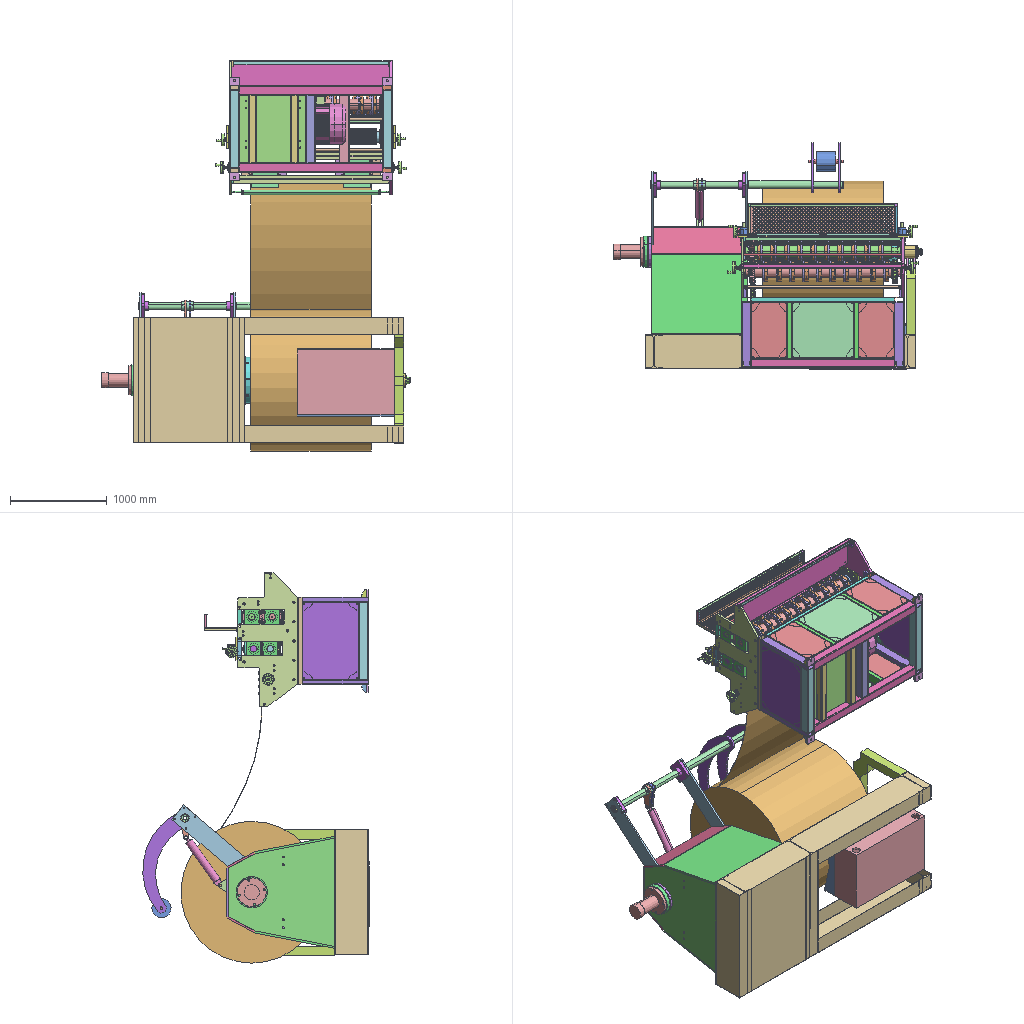Assembly | SolidWorks | 136 different items | 508 placed | box 3192 x 2340 x 4038 mm
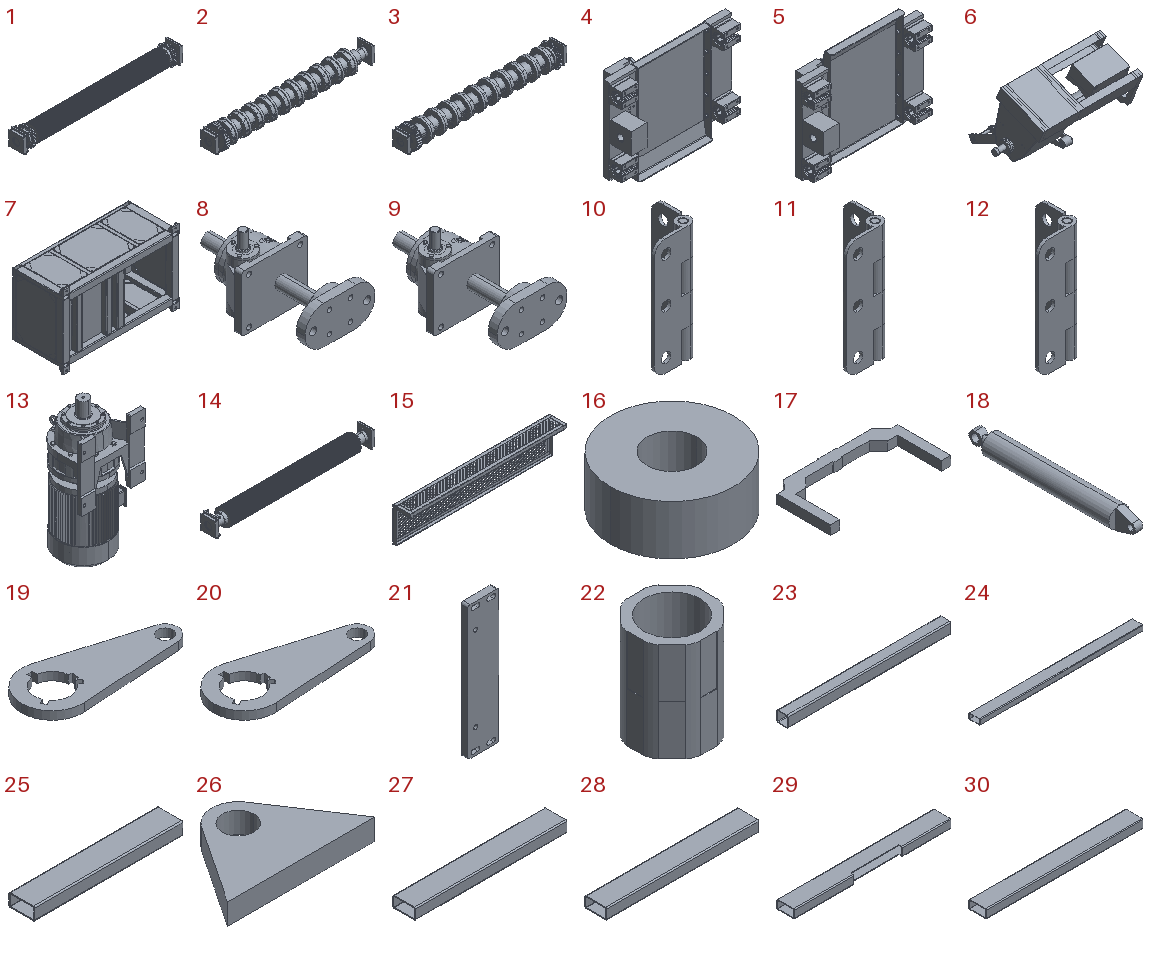Parts list (item | name | quantity | parent item | size | volume | features):
1 | (subassembly) | x1 | - | 1672 x 198.631 x 197.926 mm | 35053418 mm3 | -
2 | (subassembly) | x1 | - | 1672 x 223.661 x 223.999 mm | 30966531 mm3 | -
3 | (subassembly) | x1 | - | 1672 x 235.877 x 235.04 mm | 32005063 mm3 | -
4 | (subassembly) | x1 | - | - | 3227627 mm3 | -
5 | (subassembly) | x1 | - | - | 3227627 mm3 | -
6 | (subassembly) | x1 | - | - | 464591008 mm3 | -
7 | (subassembly) | x1 | - | 1682 x 730 x 1060 mm | 39110385 mm3 | -
8 | (subassembly) | x1 | - | 138.5 x 246 x 160 mm | 888855 mm3 | -
9 | (subassembly) | x1 | - | 138.5 x 246 x 160 mm | 888855 mm3 | -
10 | (subassembly) | x1 | - | 28.6 x 28.6 x 78 mm | 10885 mm3 | -
11 | (subassembly) | x1 | - | 28.6 x 28.6 x 78 mm | 10885 mm3 | -
12 | (subassembly) | x1 | - | 28.6 x 28.6 x 78 mm | 10885 mm3 | -
13 | (subassembly) | x1 | - | 570 x 540.12 x 1100 mm | 120754101 mm3 | -
14 | (subassembly) | x1 | - | 1672 x 169.976 x 180 mm | 33756798 mm3 | -
15 | - | x1 | - | - | 1424009 mm3 | features BaseBody 11
16 | - | x4 | in 6 | 49.497 x 49.497 x 20 mm | 32201 mm3 | features BaseBody 1
17 | - | x1 | in 6 | 1310 x 690 x 100 mm | 25394673 mm3 | features BaseBody 1
18 | - | x1 | in 6 | 80 x 654.288 x 80 mm | 2684074 mm3 | features BaseBody 1
19 | - | x1 | in 6 | 283.692 x 120 x 16 mm | 303267 mm3 | features BaseBody 1
20 | - | x1 | in 6 | 283.692 x 120 x 16 mm | 303267 mm3 | features BaseBody 1
21 | - | x2 | - | 140 x 30 x 600 mm | 2424100 mm3 | features BaseBody 1
22 | - | x1 | in 6 | 224.499 x 224.499 x 300 mm | 5216561 mm3 | features BaseBody 1
23 | - | x2 | in 7 | 1480 x 100 x 100 mm | 2716717 mm3 | features BaseBody 1
24 | - | x2 | in 7 | 1480 x 100 x 50 mm | 1650789 mm3 | features BaseBody 1
25 | - | x4 | in 7 | 580 x 100 x 50 mm | 646931 mm3 | features BaseBody 1
26 | - | x2 | in 6 | 140 x 85 x 20 mm | 126524 mm3 | features BaseBody 1
27 | - | x4 | in 7 | 680 x 100 x 50 mm | 758471 mm3 | features BaseBody 1
28 | - | x2 | in 7 | 700 x 100 x 50 mm | 780779 mm3 | features BaseBody 1
29 | - | x1 | in 7 | 900 x 100 x 50 mm | 914903 mm3 | features BaseBody 1
30 | - | x1 | in 7 | 900 x 100 x 50 mm | 1003858 mm3 | features BaseBody 1
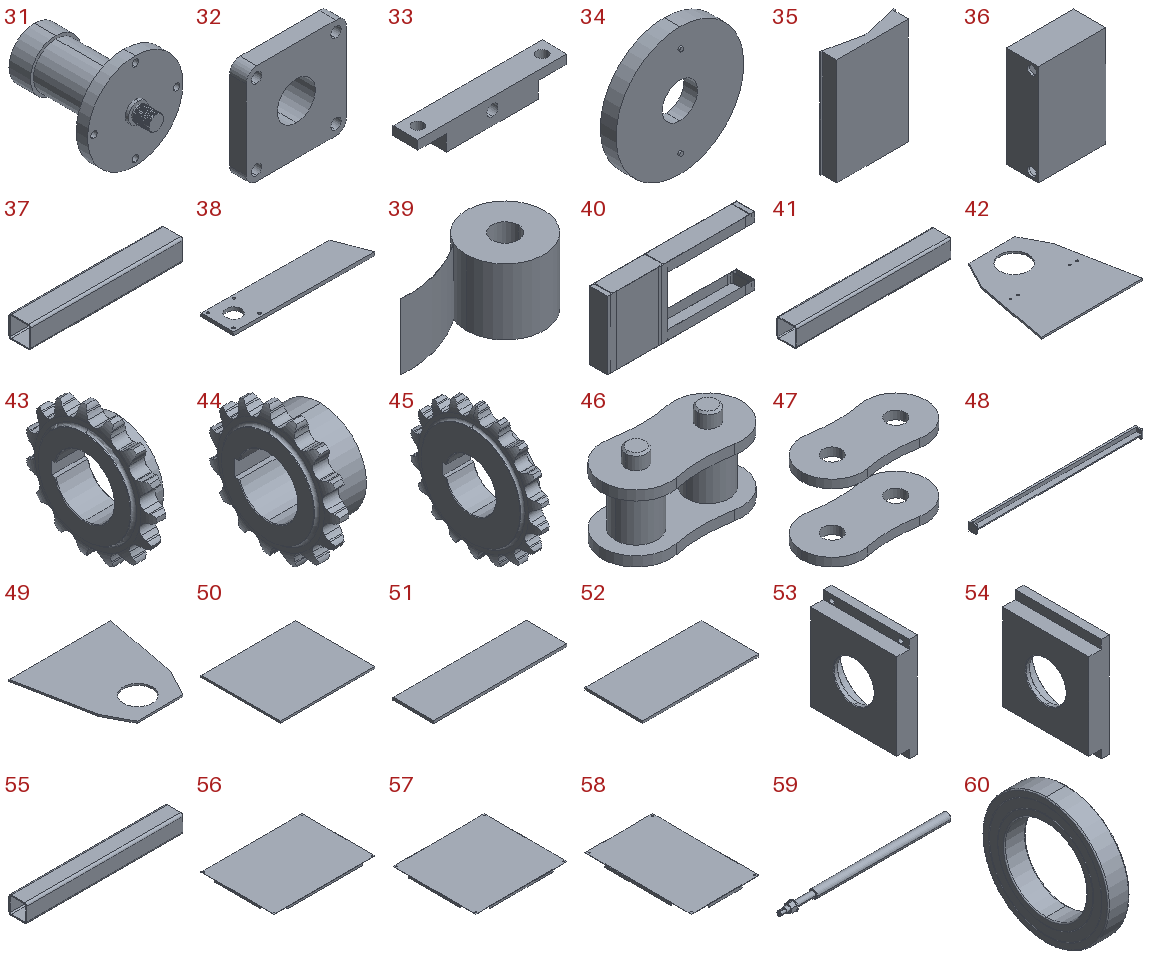31 | - | x1 | in 6 | 300 x 382.79 x 300 mm | 7334262 mm3 | features BaseBody 1
32 | - | x2 | in 6 | 193 x 74.6 x 193 mm | 1117041 mm3 | features BaseBody 1
33 | - | x2 | - | 240 x 40 x 40 mm | 271016 mm3 | features BaseBody 1
34 | - | x1 | in 6 | 325 x 45 x 325 mm | 2743003 mm3 | features BaseBody 1
35 | - | x1 | in 6 | 698.157 x 148.827 x 1000 mm | 73538698 mm3 | features BaseBody 1
36 | - | x1 | in 6 | 670 x 320 x 1000 mm | 50005072 mm3 | features BaseBody 1
37 | - | x1 | in 7 | 700 x 100 x 100 mm | 1284934 mm3 | features BaseBody 1
38 | - | x2 | in 6 | 828.827 x 200.894 x 20 mm | 2911165 mm3 | features BaseBody 1
39 | - | x1 | - | 2820 x 1466 x 1250 mm | 1870768700 mm3 | features ExtruThin 1, ICE 1
40 | - | x1 | in 6 | 2800 x 350 x 1296 mm | 23944279 mm3 | features BaseBody 1
41 | - | x2 | in 7 | 800 x 100 x 100 mm | 1468496 mm3 | features BaseBody 1
42 | - | x1 | in 6 | 1120 x 1100 x 20 mm | 17817233 mm3 | features BaseBody 1
43 | - | x2 | in 1 | 50 x 197.46 x 198.492 mm | 656500 mm3 | features BaseBody 1
44 | - | x1 | - | 80 x 197.46 x 198.492 mm | 920770 mm3 | features BaseBody 1
45 | - | x1 | in 3 | 50 x 233.402 x 236 mm | 1046718 mm3 | features BaseBody 1
46 | - | x41 | - | 74.3 x 36.2 x 50.8 mm | 46286 mm3 | features BaseBody 1
47 | - | x41 | - | 74.3 x 36.2 x 45.44 mm | 21265 mm3 | features BaseBody 2
48 | - | x2 | - | 1632 x 70 x 80 mm | 3525010 mm3 | features BaseBody 4
49 | - | x1 | in 6 | 1120 x 1100 x 20 mm | 17842366 mm3 | features BaseBody 1
50 | - | x2 | in 6 | 1000 x 836 x 20 mm | 16720000 mm3 | features BaseBody 1
51 | - | x2 | in 6 | 1000 x 305 x 20 mm | 6100000 mm3 | features BaseBody 1
52 | - | x1 | in 6 | 1000 x 500 x 20 mm | 10000000 mm3 | features BaseBody 1
53 | - | x4 | in 1, 2, 3, 14 | 36 x 150 x 180 mm | 519040 mm3 | features BaseBody 1
54 | - | x4 | in 1, 2, 3, 14 | 36 x 150 x 180 mm | 522217 mm3 | features BaseBody 1
55 | - | x2 | in 7 | 700 x 80 x 80 mm | 1004934 mm3 | features BaseBody 1
56 | - | x2 | in 7 | 795 x 575 x 15 mm | 579015 mm3 | features BaseBody 1
57 | - | x2 | in 7 | 635 x 575 x 15 mm | 463497 mm3 | features BaseBody 1
58 | - | x4 | in 7 | 365 x 575 x 15 mm | 268880 mm3 | features BaseBody 1
59 | - | x2 | - | 527.001 x 30 x 30 mm | 250409 mm3 | features BaseBody 3
60 | - | x2 | in 6 | 22 x 130 x 130 mm | 128128 mm3 | features BaseBody 26
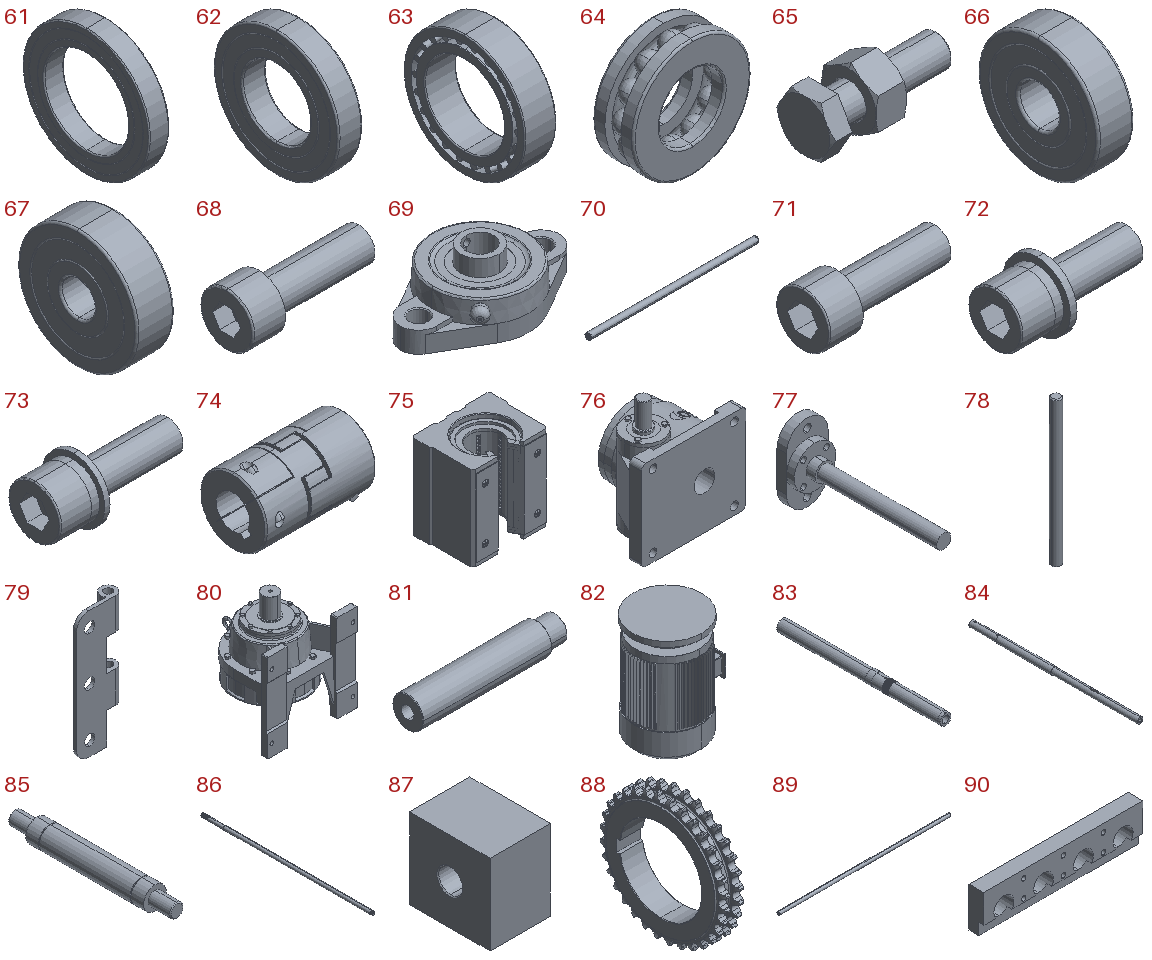61 | - | x1 | in 6 | 38 x 240 x 240 mm | 735391 mm3 | features BaseBody 27
62 | - | x8 | in 1, 2, 3, 14 | 23 x 120 x 120 mm | 144421 mm3 | features BaseBody 19
63 | - | x1 | in 6 | 67 x 260 x 260 mm | 1601339 mm3 | features BaseBody 1
64 | - | x2 | - | 35 x 12 x 35 mm | 6237 mm3 | features BaseBody 1
65 | - | x16 | in 1, 2, 3, 14 | 41.4 x 18.475 x 19.63 mm | 5747 mm3 | features BaseBody 2
66 | - | x20 | in 4, 5 | 9 x 30 x 30 mm | 4389 mm3 | features BaseBody 12
67 | - | x8 | in 4, 5 | 11 x 35 x 35 mm | 7523 mm3 | features BaseBody 11
68 | - | x44 | in 4, 5 | 33 x 13 x 13 mm | 2188 mm3 | features BaseBody 1
69 | - | x2 | - | 99 x 61 x 32.9 mm | 54285 mm3 | features BaseBody 1
70 | - | x1 | - | 1429 x 50 x 50 mm | 1432811 mm3 | features BaseBody 21
71 | - | x8 | in 4, 5 | 40 x 16 x 16 mm | 4026 mm3 | features BaseBody 1
72 | - | x8 | in 4, 5 | 40 x 20 x 20 mm | 4745 mm3 | features BaseBody 3
73 | - | x20 | in 4, 5 | 26 x 12 x 12 mm | 1103 mm3 | features BaseBody 3
74 | - | x2 | - | 66 x 41.729 x 41.508 mm | 63397 mm3 | features BaseBody 3
75 | - | x8 | in 4, 5 | 60 x 47.265 x 65 mm | 129093 mm3 | features BaseBody 5
76 | - | x2 | in 8, 9 | 122 x 84 x 160 mm | 620061 mm3 | features BaseBody 1
77 | - | x2 | in 8, 9 | 70 x 246 x 130 mm | 268794 mm3 | features BaseBody 3
78 | - | x3 | in 10, 11, 12 | 5 x 5 x 78 mm | 1528 mm3 | features BaseBody 1
79 | - | x6 | in 10, 11, 12 | 28.6 x 9.2 x 78 mm | 4679 mm3 | features BaseBody 1
80 | - | x1 | in 13 | 530 x 529 x 605 mm | 40735700 mm3 | features BaseBody 2
81 | - | x2 | - | 120 x 25 x 25 mm | 53692 mm3 | features BaseBody 1
82 | - | x1 | in 13 | 520 x 505.12 x 660 mm | 80018411 mm3 | features BaseBody 2
83 | - | x1 | in 6 | 180 x 2400 x 180 mm | 34786872 mm3 | features BaseBody 1
84 | - | x1 | in 6 | 80 x 1994 x 80 mm | 5902452 mm3 | features BaseBody 1
85 | - | x1 | in 6 | 50 x 358 x 50 mm | 578251 mm3 | features BaseBody 1
86 | - | x1 | in 6 | 55 x 2670 x 55 mm | 6167636 mm3 | features BaseBody 1
87 | - | x2 | in 4, 5 | 60 x 80 x 80 mm | 348755 mm3 | features BaseBody 1
88 | - | x1 | in 6 | 49.567 x 269.954 x 269.954 mm | 1130107 mm3 | features BaseBody 1
89 | - | x3 | - | 1632 x 30 x 30 mm | 1142665 mm3 | features BaseBody 1
90 | - | x2 | in 4, 5 | 320 x 30 x 80 mm | 527175 mm3 | features BaseBody 1
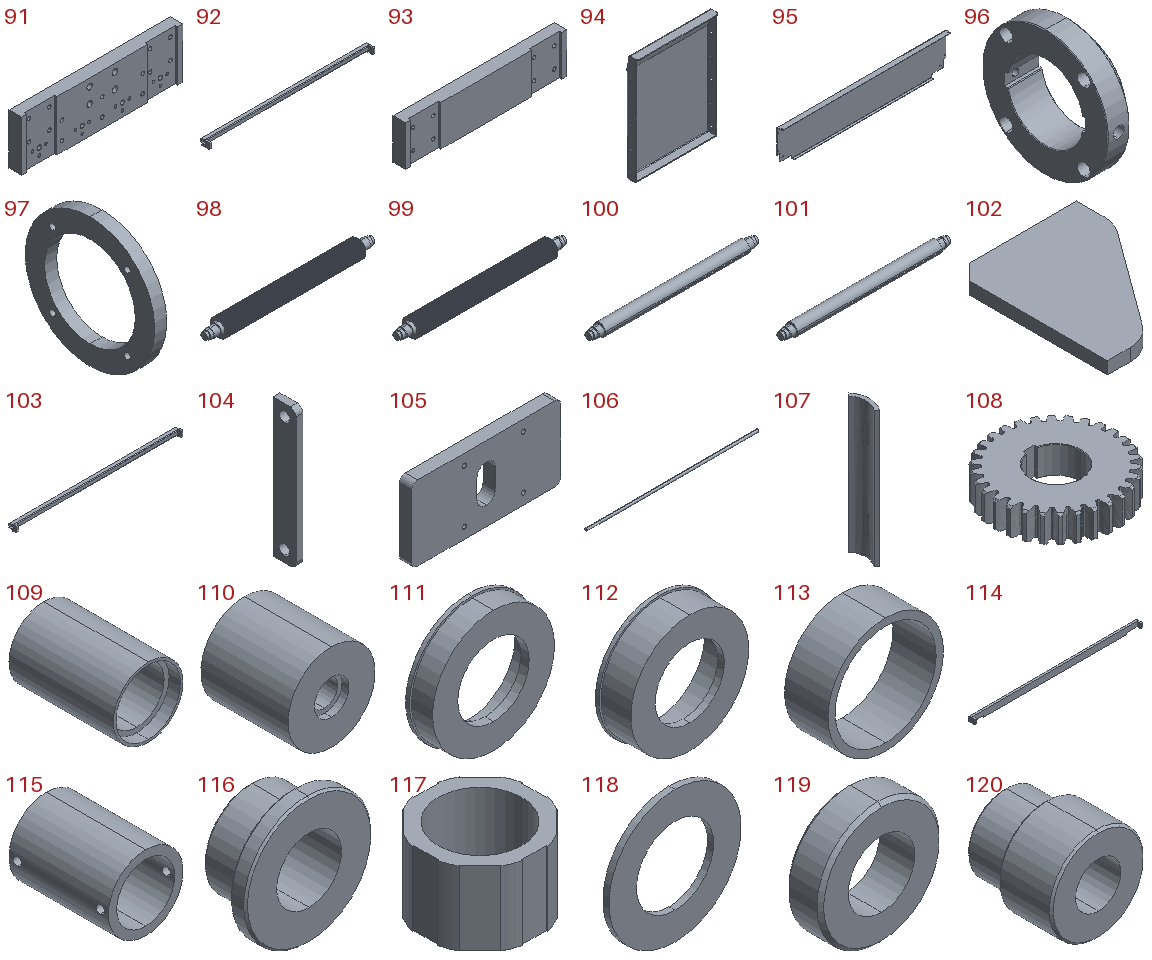91 | - | x2 | in 4, 5 | 320 x 25 x 100 mm | 683498 mm3 | features BaseBody 1
92 | - | x1 | - | 1632 x 85 x 60 mm | 797104 mm3 | features BaseBody 3
93 | - | x2 | in 4, 5 | 320 x 25 x 80 mm | 576438 mm3 | features BaseBody 1
94 | - | x2 | in 4, 5 | 280 x 38.772 x 370.012 mm | 407154 mm3 | features BaseBody 1
95 | - | x1 | - | 1680 x 53 x 340 mm | 2004466 mm3 | features BaseBody 1
96 | - | x20 | in 2, 3 | 55 x 200 x 200 mm | 776397 mm3 | features BaseBody 1
97 | - | x20 | in 2, 3 | 20 x 214 x 214 mm | 359396 mm3 | features BaseBody 1
98 | - | x1 | in 14 | 1650 x 169.976 x 169.976 mm | 32403710 mm3 | features BaseBody 2
99 | - | x1 | in 1 | 1650 x 169.976 x 169.976 mm | 32387332 mm3 | features BaseBody 2
100 | - | x1 | in 2 | 1650 x 118.322 x 120 mm | 16871280 mm3 | features BaseBody 1
101 | - | x1 | in 3 | 1650 x 118.322 x 120 mm | 16863091 mm3 | features BaseBody 1
102 | - | x32 | in 7 | 80 x 100 x 8 mm | 46944 mm3 | features BaseBody 1
103 | - | x1 | - | 1632 x 75 x 60 mm | 758697 mm3 | features BaseBody 3
104 | - | x2 | - | 12 x 40 x 240 mm | 108578 mm3 | features BaseBody 1
105 | - | x2 | - | 240 x 20 x 120 mm | 539241 mm3 | features BaseBody 1
106 | - | x1 | - | 1420 x 20 x 20 mm | 445152 mm3 | features BaseBody 1
107 | - | x4 | in 6 | 91.989 x 331.703 x 1450 mm | 19488454 mm3 | features BaseBody 1
108 | - | x2 | in 2, 3 | 224 x 223.253 x 50 mm | 1384242 mm3 | features BaseBody 1
109 | - | x1 | in 6 | 140 x 210 x 140 mm | 1063586 mm3 | features BaseBody 1
110 | - | x1 | in 6 | 200 x 200 x 200 mm | 5647327 mm3 | features BaseBody 1
111 | - | x1 | in 6 | 325 x 65 x 325 mm | 2579149 mm3 | features BaseBody 1
112 | - | x1 | in 6 | 325 x 90 x 325 mm | 2757533 mm3 | features BaseBody 1
113 | - | x1 | in 6 | 80 x 30 x 80 mm | 35343 mm3 | features BaseBody 1
114 | - | x1 | - | 1632 x 60 x 60 mm | 1939285 mm3 | features BaseBody 3
115 | - | x1 | in 6 | 90 x 120 x 90 mm | 298445 mm3 | features BaseBody 1
116 | - | x1 | in 6 | 95 x 44 x 95 mm | 126129 mm3 | features BaseBody 1
117 | - | x1 | in 6 | 224.499 x 224.499 x 150 mm | 2556210 mm3 | features BaseBody 1
118 | - | x1 | in 6 | 325 x 20 x 325 mm | 819858 mm3 | features BaseBody 1
119 | - | x1 | in 6 | 70 x 20 x 70 mm | 53424 mm3 | features BaseBody 1
120 | - | x1 | in 6 | 95 x 95 x 95 mm | 407029 mm3 | features BaseBody 1
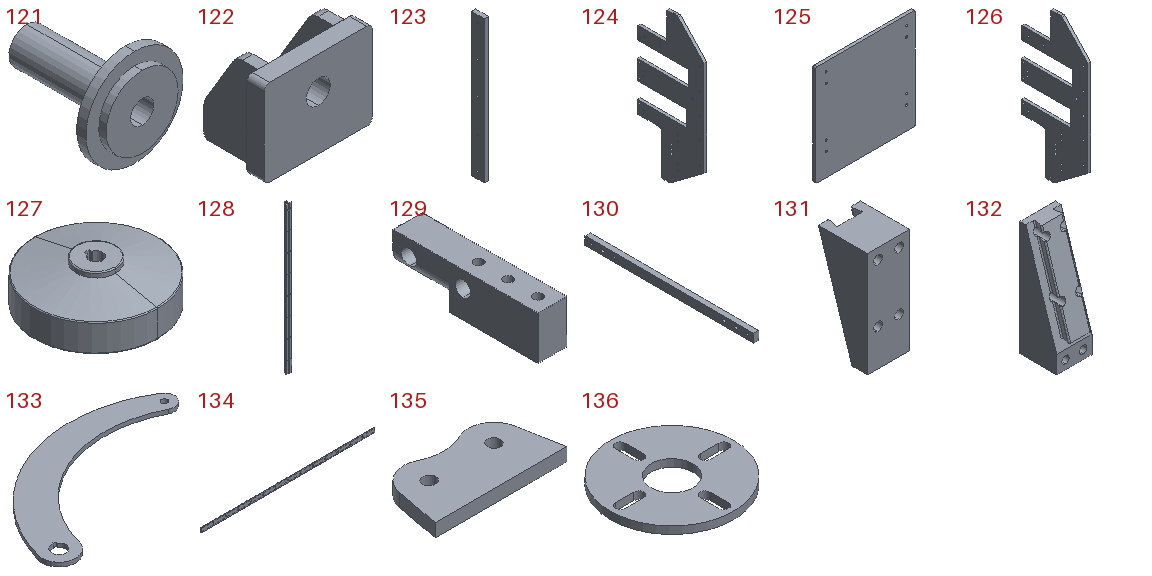121 | - | x1 | in 6 | 230 x 273 x 230 mm | 2031428 mm3 | features BaseBody 1
122 | - | x4 | in 7 | 100 x 66 x 80 mm | 186311 mm3 | features BaseBody 3
123 | - | x2 | - | 25 x 80 x 880 mm | 1740758 mm3 | features BaseBody 1
124 | - | x1 | - | 24 x 620 x 1385 mm | 11472321 mm3 | features BaseBody 1
125 | - | x1 | in 7 | 690 x 20 x 700 mm | 9633653 mm3 | features BaseBody 1
126 | - | x1 | - | 24 x 620 x 1385 mm | 11472321 mm3 | features BaseBody 1
127 | - | x4 | - | 125 x 126.49 x 97 mm | 263247 mm3 | features BaseBody 1
128 | - | x2 | - | 55 x 45.5 x 1580 mm | 1553379 mm3 | features BaseBody 1
129 | - | x4 | in 6 | 40 x 200 x 60 mm | 371568 mm3 | features BaseBody 1
130 | - | x4 | in 6 | 30 x 998 x 50 mm | 1456144 mm3 | features BaseBody 1
131 | - | x8 | in 6 | 60 x 70 x 150 mm | 318447 mm3 | features BaseBody 1
132 | - | x8 | in 6 | 60 x 72.691 x 195 mm | 513448 mm3 | features BaseBody 1
133 | - | x2 | in 6 | 1021 x 595.414 x 20 mm | 3303103 mm3 | features BaseBody 1
134 | - | x1 | - | 1400 x 1 x 38 mm | 53164 mm3 | features BaseBody 1
135 | - | x2 | in 6 | 200 x 98.946 x 20 mm | 325794 mm3 | features BaseBody 1
136 | - | x1 | in 6 | 500 x 500 x 30 mm | 4699230 mm3 | features BaseBody 1
Mates (type | each side: item.copy, entity, surface, feature):
InPlace | 39.1 plane | assembly plane